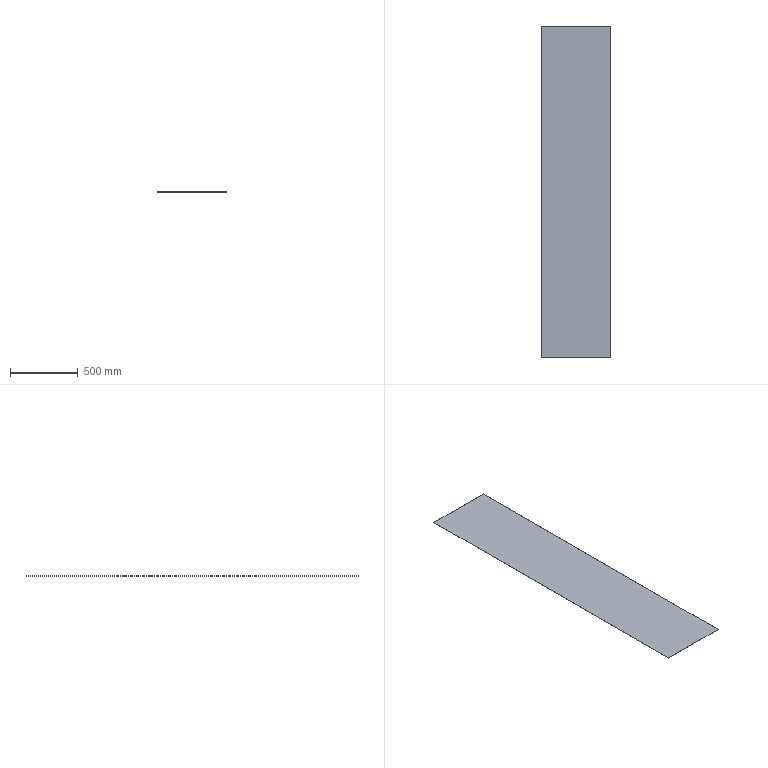Part | SolidWorks | features FlatPattern 1, SMBaseFlange 1, SheetMetal 1 | 1 solid | 6 faces | box 514 x 2442 x 1.2 mm | volume 1506226 mm3 | plane 6
STEP:
#1=CARTESIAN_POINT('',(-20.331,2413.243,0.));
#2=VERTEX_POINT('',#1);
#3=CARTESIAN_POINT('',(-20.331,-28.757,0.));
#4=VERTEX_POINT('',#3);
#5=CARTESIAN_POINT('',(-20.331,-28.757,0.));
#6=DIRECTION('',(0.,-1.,0.));
#7=VECTOR('',#6,1000.);
#8=LINE('',#5,#7);
#9=EDGE_CURVE('',#2,#4,#8,.T.);
#10=ORIENTED_EDGE('',*,*,#9,.F.);
#11=CARTESIAN_POINT('',(-20.331,2413.243,-1.2));
#12=VERTEX_POINT('',#11);
#13=CARTESIAN_POINT('',(-20.331,2413.243,-1.2));
#14=DIRECTION('',(0.,0.,1.));
#15=VECTOR('',#14,1000.);
#16=LINE('',#13,#15);
#17=EDGE_CURVE('',#12,#2,#16,.T.);
#18=ORIENTED_EDGE('',*,*,#17,.F.);
#19=CARTESIAN_POINT('',(-20.331,-28.757,-1.2));
#20=VERTEX_POINT('',#19);
#21=CARTESIAN_POINT('',(-20.331,-28.757,-1.2));
#22=DIRECTION('',(0.,-1.,0.));
#23=VECTOR('',#22,1000.);
#24=LINE('',#21,#23);
#25=EDGE_CURVE('',#12,#20,#24,.T.);
#26=ORIENTED_EDGE('',*,*,#25,.T.);
#27=CARTESIAN_POINT('',(-20.331,-28.757,-1.2));
#28=DIRECTION('',(0.,0.,1.));
#29=VECTOR('',#28,1000.);
#30=LINE('',#27,#29);
#31=EDGE_CURVE('',#20,#4,#30,.T.);
#32=ORIENTED_EDGE('',*,*,#31,.T.);
#33=EDGE_LOOP('',(#10,#18,#26,#32));
#34=FACE_OUTER_BOUND('',#33,.T.);
#35=CARTESIAN_POINT('',(-20.331,-28.757,-1.2));
#36=DIRECTION('',(-1.,0.,0.));
#37=DIRECTION('',(0.,0.,1.));
#38=AXIS2_PLACEMENT_3D('',#35,#36,#37);
#39=PLANE('',#38);
#40=ADVANCED_FACE('',(#34),#39,.T.);
#41=CARTESIAN_POINT('',(493.669,2413.243,0.));
#42=VERTEX_POINT('',#41);
#43=CARTESIAN_POINT('',(-20.331,2413.243,0.));
#44=DIRECTION('',(-1.,0.,0.));
#45=VECTOR('',#44,1000.);
#46=LINE('',#43,#45);
#47=EDGE_CURVE('',#42,#2,#46,.T.);
#48=ORIENTED_EDGE('',*,*,#47,.F.);
#49=CARTESIAN_POINT('',(493.669,2413.243,-1.2));
#50=VERTEX_POINT('',#49);
#51=CARTESIAN_POINT('',(493.669,2413.243,-1.2));
#52=DIRECTION('',(0.,0.,1.));
#53=VECTOR('',#52,1000.);
#54=LINE('',#51,#53);
#55=EDGE_CURVE('',#50,#42,#54,.T.);
#56=ORIENTED_EDGE('',*,*,#55,.F.);
#57=CARTESIAN_POINT('',(-20.331,2413.243,-1.2));
#58=DIRECTION('',(-1.,0.,0.));
#59=VECTOR('',#58,1000.);
#60=LINE('',#57,#59);
#61=EDGE_CURVE('',#50,#12,#60,.T.);
#62=ORIENTED_EDGE('',*,*,#61,.T.);
#63=ORIENTED_EDGE('',*,*,#17,.T.);
#64=EDGE_LOOP('',(#48,#56,#62,#63));
#65=FACE_OUTER_BOUND('',#64,.T.);
#66=CARTESIAN_POINT('',(-20.331,2413.243,-1.2));
#67=DIRECTION('',(0.,1.,0.));
#68=DIRECTION('',(0.,0.,1.));
#69=AXIS2_PLACEMENT_3D('',#66,#67,#68);
#70=PLANE('',#69);
#71=ADVANCED_FACE('',(#65),#70,.T.);
#72=CARTESIAN_POINT('',(493.669,-28.757,0.));
#73=VERTEX_POINT('',#72);
#74=CARTESIAN_POINT('',(493.669,-28.757,0.));
#75=DIRECTION('',(0.,1.,0.));
#76=VECTOR('',#75,1000.);
#77=LINE('',#74,#76);
#78=EDGE_CURVE('',#73,#42,#77,.T.);
#79=ORIENTED_EDGE('',*,*,#78,.F.);
#80=CARTESIAN_POINT('',(493.669,-28.757,-1.2));
#81=VERTEX_POINT('',#80);
#82=CARTESIAN_POINT('',(493.669,-28.757,-1.2));
#83=DIRECTION('',(0.,0.,1.));
#84=VECTOR('',#83,1000.);
#85=LINE('',#82,#84);
#86=EDGE_CURVE('',#81,#73,#85,.T.);
#87=ORIENTED_EDGE('',*,*,#86,.F.);
#88=CARTESIAN_POINT('',(493.669,-28.757,-1.2));
#89=DIRECTION('',(0.,1.,0.));
#90=VECTOR('',#89,1000.);
#91=LINE('',#88,#90);
#92=EDGE_CURVE('',#81,#50,#91,.T.);
#93=ORIENTED_EDGE('',*,*,#92,.T.);
#94=ORIENTED_EDGE('',*,*,#55,.T.);
#95=EDGE_LOOP('',(#79,#87,#93,#94));
#96=FACE_OUTER_BOUND('',#95,.T.);
#97=CARTESIAN_POINT('',(493.669,-28.757,-1.2));
#98=DIRECTION('',(1.,0.,0.));
#99=DIRECTION('',(0.,0.,-1.));
#100=AXIS2_PLACEMENT_3D('',#97,#98,#99);
#101=PLANE('',#100);
#102=ADVANCED_FACE('',(#96),#101,.T.);
#103=CARTESIAN_POINT('',(-20.331,-28.757,0.));
#104=DIRECTION('',(1.,0.,0.));
#105=VECTOR('',#104,1000.);
#106=LINE('',#103,#105);
#107=EDGE_CURVE('',#4,#73,#106,.T.);
#108=ORIENTED_EDGE('',*,*,#107,.F.);
#109=ORIENTED_EDGE('',*,*,#31,.F.);
#110=CARTESIAN_POINT('',(-20.331,-28.757,-1.2));
#111=DIRECTION('',(1.,0.,0.));
#112=VECTOR('',#111,1000.);
#113=LINE('',#110,#112);
#114=EDGE_CURVE('',#20,#81,#113,.T.);
#115=ORIENTED_EDGE('',*,*,#114,.T.);
#116=ORIENTED_EDGE('',*,*,#86,.T.);
#117=EDGE_LOOP('',(#108,#109,#115,#116));
#118=FACE_OUTER_BOUND('',#117,.T.);
#119=CARTESIAN_POINT('',(-20.331,-28.757,-1.2));
#120=DIRECTION('',(0.,-1.,0.));
#121=DIRECTION('',(0.,0.,-1.));
#122=AXIS2_PLACEMENT_3D('',#119,#120,#121);
#123=PLANE('',#122);
#124=ADVANCED_FACE('',(#118),#123,.T.);
#125=ORIENTED_EDGE('',*,*,#25,.F.);
#126=ORIENTED_EDGE('',*,*,#61,.F.);
#127=ORIENTED_EDGE('',*,*,#92,.F.);
#128=ORIENTED_EDGE('',*,*,#114,.F.);
#129=EDGE_LOOP('',(#125,#126,#127,#128));
#130=FACE_OUTER_BOUND('',#129,.T.);
#131=CARTESIAN_POINT('',(0.,0.,-1.2));
#132=DIRECTION('',(0.,0.,-1.));
#133=DIRECTION('',(-1.,0.,0.));
#134=AXIS2_PLACEMENT_3D('',#131,#132,#133);
#135=PLANE('',#134);
#136=ADVANCED_FACE('',(#130),#135,.T.);
#137=ORIENTED_EDGE('',*,*,#9,.T.);
#138=ORIENTED_EDGE('',*,*,#107,.T.);
#139=ORIENTED_EDGE('',*,*,#78,.T.);
#140=ORIENTED_EDGE('',*,*,#47,.T.);
#141=EDGE_LOOP('',(#137,#138,#139,#140));
#142=FACE_OUTER_BOUND('',#141,.T.);
#143=CARTESIAN_POINT('',(0.,0.,0.));
#144=DIRECTION('',(0.,0.,-1.));
#145=DIRECTION('',(-1.,0.,0.));
#146=AXIS2_PLACEMENT_3D('',#143,#144,#145);
#147=PLANE('',#146);
#148=ADVANCED_FACE('',(#142),#147,.F.);
#149=CLOSED_SHELL('',(#40,#71,#102,#124,#136,#148));
#150=MANIFOLD_SOLID_BREP('',#149);
#151=CARTESIAN_POINT('',(0.,0.,0.));
#152=DIRECTION('',(0.,0.,1.));
#153=DIRECTION('',(1.,0.,0.));
#154=AXIS2_PLACEMENT_3D('',#151,#152,#153);
#155=(LENGTH_UNIT()NAMED_UNIT(*)SI_UNIT(.MILLI.,.METRE.));
#156=UNCERTAINTY_MEASURE_WITH_UNIT(LENGTH_MEASURE(0.00001),#155,'','');
#157=(NAMED_UNIT(*)PLANE_ANGLE_UNIT()SI_UNIT($,.RADIAN.));
#158=(NAMED_UNIT(*)SI_UNIT($,.STERADIAN.)SOLID_ANGLE_UNIT());
#159=(GEOMETRIC_REPRESENTATION_CONTEXT(3)GLOBAL_UNCERTAINTY_ASSIGNED_CONTEXT((#156))GLOBAL_UNIT_ASSIGNED_CONTEXT((#155,#157,#158))REPRESENTATION_CONTEXT('',''));
#160=ADVANCED_BREP_SHAPE_REPRESENTATION('',(#150,#154),#159);